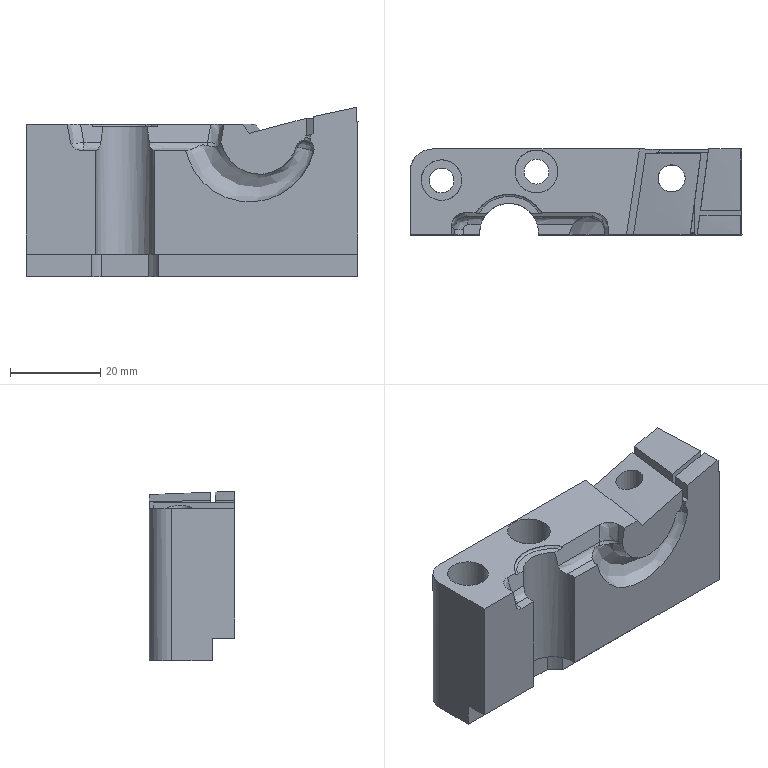Part | STEP file | P011002M009-000 | 1 solid | 60 faces | box 73.5 x 19 x 37.504 mm | volume 38643 mm3 | spline 31 | plane 16 | cylinder 10 | other 1 | cone 1 | torus 1 | commonest cylinder face diameters 5.5 x2 17.5 x2 6 x1 9 x1 9.5 x1 10 x1